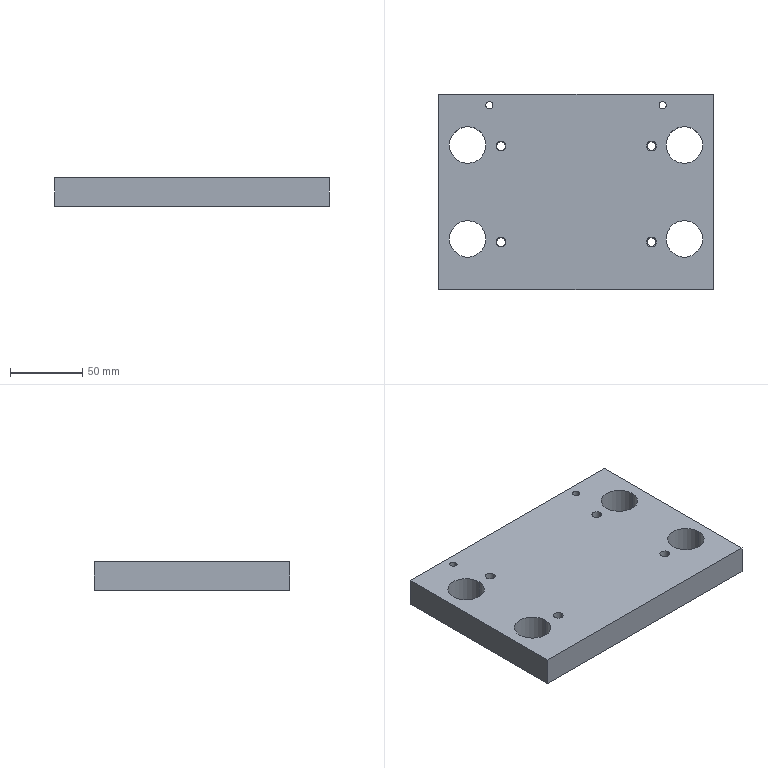Part | SolidWorks | features HoleWzd 2, Extrusion 1 | 1 solid | 34 faces | box 190 x 135 x 20 mm | volume 469337 mm3 | cylinder 20 | cone 8 | plane 6 | commonest cylinder face diameters 6.8 x8 25.224 x8 5 x4
STEP:
#1=CARTESIAN_POINT('',(-55.367,31.821,0.25));
#2=VERTEX_POINT('',#1);
#3=CARTESIAN_POINT('',(-48.567,31.821,0.25));
#4=VERTEX_POINT('',#3);
#5=CARTESIAN_POINT('',(-51.967,31.821,0.25));
#6=DIRECTION('',(0.,0.,1.));
#7=DIRECTION('',(1.,0.,0.));
#8=AXIS2_PLACEMENT_3D('',#5,#6,#7);
#9=CIRCLE('',#8,3.4);
#10=EDGE_CURVE('',#2,#4,#9,.T.);
#11=ORIENTED_EDGE('',*,*,#10,.F.);
#12=CARTESIAN_POINT('',(-55.367,31.821,20.));
#13=VERTEX_POINT('',#12);
#14=CARTESIAN_POINT('',(-55.367,31.821,20.));
#15=DIRECTION('',(0.,0.,1.));
#16=VECTOR('',#15,1000.);
#17=LINE('',#14,#16);
#18=EDGE_CURVE('',#2,#13,#17,.T.);
#19=ORIENTED_EDGE('',*,*,#18,.T.);
#20=CARTESIAN_POINT('',(-48.567,31.821,20.));
#21=VERTEX_POINT('',#20);
#22=CARTESIAN_POINT('',(-51.967,31.821,20.));
#23=DIRECTION('',(0.,0.,1.));
#24=DIRECTION('',(1.,0.,0.));
#25=AXIS2_PLACEMENT_3D('',#22,#23,#24);
#26=CIRCLE('',#25,3.4);
#27=EDGE_CURVE('',#13,#21,#26,.T.);
#28=ORIENTED_EDGE('',*,*,#27,.T.);
#29=CARTESIAN_POINT('',(-48.567,31.821,20.));
#30=DIRECTION('',(0.,0.,1.));
#31=VECTOR('',#30,1000.);
#32=LINE('',#29,#31);
#33=EDGE_CURVE('',#4,#21,#32,.T.);
#34=ORIENTED_EDGE('',*,*,#33,.F.);
#35=EDGE_LOOP('',(#11,#19,#28,#34));
#36=FACE_OUTER_BOUND('',#35,.T.);
#37=CARTESIAN_POINT('',(-51.967,31.821,20.));
#38=DIRECTION('',(0.,0.,1.));
#39=DIRECTION('',(1.,0.,0.));
#40=AXIS2_PLACEMENT_3D('',#37,#38,#39);
#41=CYLINDRICAL_SURFACE('',#40,3.4);
#42=ADVANCED_FACE('',(#36),#41,.F.);
#43=CARTESIAN_POINT('',(-54.951,31.821,0.));
#44=VERTEX_POINT('',#43);
#45=CARTESIAN_POINT('',(-48.984,31.821,0.));
#46=VERTEX_POINT('',#45);
#47=CARTESIAN_POINT('',(-51.967,31.821,0.));
#48=DIRECTION('',(0.,0.,1.));
#49=DIRECTION('',(1.,0.,0.));
#50=AXIS2_PLACEMENT_3D('',#47,#48,#49);
#51=CIRCLE('',#50,2.984);
#52=EDGE_CURVE('',#44,#46,#51,.T.);
#53=ORIENTED_EDGE('',*,*,#52,.F.);
#54=CARTESIAN_POINT('',(-55.367,31.821,0.25));
#55=DIRECTION('',(-0.8572,0.,0.515));
#56=VECTOR('',#55,1000.);
#57=LINE('',#54,#56);
#58=EDGE_CURVE('',#44,#2,#57,.T.);
#59=ORIENTED_EDGE('',*,*,#58,.T.);
#60=ORIENTED_EDGE('',*,*,#10,.T.);
#61=CARTESIAN_POINT('',(-48.567,31.821,0.25));
#62=DIRECTION('',(0.8572,0.,0.515));
#63=VECTOR('',#62,1000.);
#64=LINE('',#61,#63);
#65=EDGE_CURVE('',#46,#4,#64,.T.);
#66=ORIENTED_EDGE('',*,*,#65,.F.);
#67=EDGE_LOOP('',(#53,#59,#60,#66));
#68=FACE_OUTER_BOUND('',#67,.T.);
#69=CARTESIAN_POINT('',(-51.967,31.821,0.25));
#70=DIRECTION('',(0.,0.,1.));
#71=DIRECTION('',(1.,0.,0.));
#72=AXIS2_PLACEMENT_3D('',#69,#70,#71);
#73=CONICAL_SURFACE('',#72,3.4,1.03);
#74=ADVANCED_FACE('',(#68),#73,.F.);
#75=CARTESIAN_POINT('',(-55.367,-34.623,0.25));
#76=VERTEX_POINT('',#75);
#77=CARTESIAN_POINT('',(-48.567,-34.623,0.25));
#78=VERTEX_POINT('',#77);
#79=CARTESIAN_POINT('',(-51.967,-34.623,0.25));
#80=DIRECTION('',(0.,0.,1.));
#81=DIRECTION('',(1.,0.,0.));
#82=AXIS2_PLACEMENT_3D('',#79,#80,#81);
#83=CIRCLE('',#82,3.4);
#84=EDGE_CURVE('',#76,#78,#83,.T.);
#85=ORIENTED_EDGE('',*,*,#84,.F.);
#86=CARTESIAN_POINT('',(-55.367,-34.623,20.));
#87=VERTEX_POINT('',#86);
#88=CARTESIAN_POINT('',(-55.367,-34.623,20.));
#89=DIRECTION('',(0.,0.,1.));
#90=VECTOR('',#89,1000.);
#91=LINE('',#88,#90);
#92=EDGE_CURVE('',#76,#87,#91,.T.);
#93=ORIENTED_EDGE('',*,*,#92,.T.);
#94=CARTESIAN_POINT('',(-48.567,-34.623,20.));
#95=VERTEX_POINT('',#94);
#96=CARTESIAN_POINT('',(-51.967,-34.623,20.));
#97=DIRECTION('',(0.,0.,1.));
#98=DIRECTION('',(1.,0.,0.));
#99=AXIS2_PLACEMENT_3D('',#96,#97,#98);
#100=CIRCLE('',#99,3.4);
#101=EDGE_CURVE('',#87,#95,#100,.T.);
#102=ORIENTED_EDGE('',*,*,#101,.T.);
#103=CARTESIAN_POINT('',(-48.567,-34.623,20.));
#104=DIRECTION('',(0.,0.,1.));
#105=VECTOR('',#104,1000.);
#106=LINE('',#103,#105);
#107=EDGE_CURVE('',#78,#95,#106,.T.);
#108=ORIENTED_EDGE('',*,*,#107,.F.);
#109=EDGE_LOOP('',(#85,#93,#102,#108));
#110=FACE_OUTER_BOUND('',#109,.T.);
#111=CARTESIAN_POINT('',(-51.967,-34.623,20.));
#112=DIRECTION('',(0.,0.,1.));
#113=DIRECTION('',(1.,0.,0.));
#114=AXIS2_PLACEMENT_3D('',#111,#112,#113);
#115=CYLINDRICAL_SURFACE('',#114,3.4);
#116=ADVANCED_FACE('',(#110),#115,.F.);
#117=CARTESIAN_POINT('',(-54.951,-34.623,0.));
#118=VERTEX_POINT('',#117);
#119=CARTESIAN_POINT('',(-48.984,-34.623,0.));
#120=VERTEX_POINT('',#119);
#121=CARTESIAN_POINT('',(-51.967,-34.623,0.));
#122=DIRECTION('',(0.,0.,1.));
#123=DIRECTION('',(1.,0.,0.));
#124=AXIS2_PLACEMENT_3D('',#121,#122,#123);
#125=CIRCLE('',#124,2.984);
#126=EDGE_CURVE('',#118,#120,#125,.T.);
#127=ORIENTED_EDGE('',*,*,#126,.F.);
#128=CARTESIAN_POINT('',(-55.367,-34.623,0.25));
#129=DIRECTION('',(-0.8572,0.,0.515));
#130=VECTOR('',#129,1000.);
#131=LINE('',#128,#130);
#132=EDGE_CURVE('',#118,#76,#131,.T.);
#133=ORIENTED_EDGE('',*,*,#132,.T.);
#134=ORIENTED_EDGE('',*,*,#84,.T.);
#135=CARTESIAN_POINT('',(-48.567,-34.623,0.25));
#136=DIRECTION('',(0.8572,0.,0.515));
#137=VECTOR('',#136,1000.);
#138=LINE('',#135,#137);
#139=EDGE_CURVE('',#120,#78,#138,.T.);
#140=ORIENTED_EDGE('',*,*,#139,.F.);
#141=EDGE_LOOP('',(#127,#133,#134,#140));
#142=FACE_OUTER_BOUND('',#141,.T.);
#143=CARTESIAN_POINT('',(-51.967,-34.623,0.25));
#144=DIRECTION('',(0.,0.,1.));
#145=DIRECTION('',(1.,0.,0.));
#146=AXIS2_PLACEMENT_3D('',#143,#144,#145);
#147=CONICAL_SURFACE('',#146,3.4,1.03);
#148=ADVANCED_FACE('',(#142),#147,.F.);
#149=CARTESIAN_POINT('',(48.834,-34.623,0.25));
#150=VERTEX_POINT('',#149);
#151=CARTESIAN_POINT('',(55.634,-34.623,0.25));
#152=VERTEX_POINT('',#151);
#153=CARTESIAN_POINT('',(52.234,-34.623,0.25));
#154=DIRECTION('',(0.,0.,1.));
#155=DIRECTION('',(1.,0.,0.));
#156=AXIS2_PLACEMENT_3D('',#153,#154,#155);
#157=CIRCLE('',#156,3.4);
#158=EDGE_CURVE('',#150,#152,#157,.T.);
#159=ORIENTED_EDGE('',*,*,#158,.F.);
#160=CARTESIAN_POINT('',(48.834,-34.623,20.));
#161=VERTEX_POINT('',#160);
#162=CARTESIAN_POINT('',(48.834,-34.623,20.));
#163=DIRECTION('',(0.,0.,1.));
#164=VECTOR('',#163,1000.);
#165=LINE('',#162,#164);
#166=EDGE_CURVE('',#150,#161,#165,.T.);
#167=ORIENTED_EDGE('',*,*,#166,.T.);
#168=CARTESIAN_POINT('',(55.634,-34.623,20.));
#169=VERTEX_POINT('',#168);
#170=CARTESIAN_POINT('',(52.234,-34.623,20.));
#171=DIRECTION('',(0.,0.,1.));
#172=DIRECTION('',(1.,0.,0.));
#173=AXIS2_PLACEMENT_3D('',#170,#171,#172);
#174=CIRCLE('',#173,3.4);
#175=EDGE_CURVE('',#161,#169,#174,.T.);
#176=ORIENTED_EDGE('',*,*,#175,.T.);
#177=CARTESIAN_POINT('',(55.634,-34.623,20.));
#178=DIRECTION('',(0.,0.,1.));
#179=VECTOR('',#178,1000.);
#180=LINE('',#177,#179);
#181=EDGE_CURVE('',#152,#169,#180,.T.);
#182=ORIENTED_EDGE('',*,*,#181,.F.);
#183=EDGE_LOOP('',(#159,#167,#176,#182));
#184=FACE_OUTER_BOUND('',#183,.T.);
#185=CARTESIAN_POINT('',(52.234,-34.623,20.));
#186=DIRECTION('',(0.,0.,1.));
#187=DIRECTION('',(1.,0.,0.));
#188=AXIS2_PLACEMENT_3D('',#185,#186,#187);
#189=CYLINDRICAL_SURFACE('',#188,3.4);
#190=ADVANCED_FACE('',(#184),#189,.F.);
#191=CARTESIAN_POINT('',(49.25,-34.623,0.));
#192=VERTEX_POINT('',#191);
#193=CARTESIAN_POINT('',(55.218,-34.623,0.));
#194=VERTEX_POINT('',#193);
#195=CARTESIAN_POINT('',(52.234,-34.623,0.));
#196=DIRECTION('',(0.,0.,1.));
#197=DIRECTION('',(1.,0.,0.));
#198=AXIS2_PLACEMENT_3D('',#195,#196,#197);
#199=CIRCLE('',#198,2.984);
#200=EDGE_CURVE('',#192,#194,#199,.T.);
#201=ORIENTED_EDGE('',*,*,#200,.F.);
#202=CARTESIAN_POINT('',(48.834,-34.623,0.25));
#203=DIRECTION('',(-0.8572,0.,0.515));
#204=VECTOR('',#203,1000.);
#205=LINE('',#202,#204);
#206=EDGE_CURVE('',#192,#150,#205,.T.);
#207=ORIENTED_EDGE('',*,*,#206,.T.);
#208=ORIENTED_EDGE('',*,*,#158,.T.);
#209=CARTESIAN_POINT('',(55.634,-34.623,0.25));
#210=DIRECTION('',(0.8572,0.,0.515));
#211=VECTOR('',#210,1000.);
#212=LINE('',#209,#211);
#213=EDGE_CURVE('',#194,#152,#212,.T.);
#214=ORIENTED_EDGE('',*,*,#213,.F.);
#215=EDGE_LOOP('',(#201,#207,#208,#214));
#216=FACE_OUTER_BOUND('',#215,.T.);
#217=CARTESIAN_POINT('',(52.234,-34.623,0.25));
#218=DIRECTION('',(0.,0.,1.));
#219=DIRECTION('',(1.,0.,0.));
#220=AXIS2_PLACEMENT_3D('',#217,#218,#219);
#221=CONICAL_SURFACE('',#220,3.4,1.03);
#222=ADVANCED_FACE('',(#216),#221,.F.);
#223=CARTESIAN_POINT('',(48.834,31.821,0.25));
#224=VERTEX_POINT('',#223);
#225=CARTESIAN_POINT('',(55.634,31.821,0.25));
#226=VERTEX_POINT('',#225);
#227=CARTESIAN_POINT('',(52.234,31.821,0.25));
#228=DIRECTION('',(0.,0.,1.));
#229=DIRECTION('',(1.,0.,0.));
#230=AXIS2_PLACEMENT_3D('',#227,#228,#229);
#231=CIRCLE('',#230,3.4);
#232=EDGE_CURVE('',#224,#226,#231,.T.);
#233=ORIENTED_EDGE('',*,*,#232,.F.);
#234=CARTESIAN_POINT('',(48.834,31.821,20.));
#235=VERTEX_POINT('',#234);
#236=CARTESIAN_POINT('',(48.834,31.821,20.));
#237=DIRECTION('',(0.,0.,1.));
#238=VECTOR('',#237,1000.);
#239=LINE('',#236,#238);
#240=EDGE_CURVE('',#224,#235,#239,.T.);
#241=ORIENTED_EDGE('',*,*,#240,.T.);
#242=CARTESIAN_POINT('',(55.634,31.821,20.));
#243=VERTEX_POINT('',#242);
#244=CARTESIAN_POINT('',(52.234,31.821,20.));
#245=DIRECTION('',(0.,0.,1.));
#246=DIRECTION('',(1.,0.,0.));
#247=AXIS2_PLACEMENT_3D('',#244,#245,#246);
#248=CIRCLE('',#247,3.4);
#249=EDGE_CURVE('',#235,#243,#248,.T.);
#250=ORIENTED_EDGE('',*,*,#249,.T.);
#251=CARTESIAN_POINT('',(55.634,31.821,20.));
#252=DIRECTION('',(0.,0.,1.));
#253=VECTOR('',#252,1000.);
#254=LINE('',#251,#253);
#255=EDGE_CURVE('',#226,#243,#254,.T.);
#256=ORIENTED_EDGE('',*,*,#255,.F.);
#257=EDGE_LOOP('',(#233,#241,#250,#256));
#258=FACE_OUTER_BOUND('',#257,.T.);
#259=CARTESIAN_POINT('',(52.234,31.821,20.));
#260=DIRECTION('',(0.,0.,1.));
#261=DIRECTION('',(1.,0.,0.));
#262=AXIS2_PLACEMENT_3D('',#259,#260,#261);
#263=CYLINDRICAL_SURFACE('',#262,3.4);
#264=ADVANCED_FACE('',(#258),#263,.F.);
#265=CARTESIAN_POINT('',(49.25,31.821,0.));
#266=VERTEX_POINT('',#265);
#267=CARTESIAN_POINT('',(55.218,31.821,0.));
#268=VERTEX_POINT('',#267);
#269=CARTESIAN_POINT('',(52.234,31.821,0.));
#270=DIRECTION('',(0.,0.,1.));
#271=DIRECTION('',(1.,0.,0.));
#272=AXIS2_PLACEMENT_3D('',#269,#270,#271);
#273=CIRCLE('',#272,2.984);
#274=EDGE_CURVE('',#266,#268,#273,.T.);
#275=ORIENTED_EDGE('',*,*,#274,.F.);
#276=CARTESIAN_POINT('',(48.834,31.821,0.25));
#277=DIRECTION('',(-0.8572,0.,0.515));
#278=VECTOR('',#277,1000.);
#279=LINE('',#276,#278);
#280=EDGE_CURVE('',#266,#224,#279,.T.);
#281=ORIENTED_EDGE('',*,*,#280,.T.);
#282=ORIENTED_EDGE('',*,*,#232,.T.);
#283=CARTESIAN_POINT('',(55.634,31.821,0.25));
#284=DIRECTION('',(0.8572,0.,0.515));
#285=VECTOR('',#284,1000.);
#286=LINE('',#283,#285);
#287=EDGE_CURVE('',#268,#226,#286,.T.);
#288=ORIENTED_EDGE('',*,*,#287,.F.);
#289=EDGE_LOOP('',(#275,#281,#282,#288));
#290=FACE_OUTER_BOUND('',#289,.T.);
#291=CARTESIAN_POINT('',(52.234,31.821,0.25));
#292=DIRECTION('',(0.,0.,1.));
#293=DIRECTION('',(1.,0.,0.));
#294=AXIS2_PLACEMENT_3D('',#291,#292,#293);
#295=CONICAL_SURFACE('',#294,3.4,1.03);
#296=ADVANCED_FACE('',(#290),#295,.F.);
#297=CARTESIAN_POINT('',(62.5,60.,20.));
#298=VERTEX_POINT('',#297);
#299=CARTESIAN_POINT('',(57.5,60.,20.));
#300=VERTEX_POINT('',#299);
#301=CARTESIAN_POINT('',(60.,60.,20.));
#302=DIRECTION('',(0.,0.,-1.));
#303=DIRECTION('',(-1.,0.,0.));
#304=AXIS2_PLACEMENT_3D('',#301,#302,#303);
#305=CIRCLE('',#304,2.5);
#306=EDGE_CURVE('',#298,#300,#305,.T.);
#307=ORIENTED_EDGE('',*,*,#306,.F.);
#308=CARTESIAN_POINT('',(62.5,60.,0.));
#309=VERTEX_POINT('',#308);
#310=CARTESIAN_POINT('',(62.5,60.,0.));
#311=DIRECTION('',(0.,0.,-1.));
#312=VECTOR('',#311,1000.);
#313=LINE('',#310,#312);
#314=EDGE_CURVE('',#298,#309,#313,.T.);
#315=ORIENTED_EDGE('',*,*,#314,.T.);
#316=CARTESIAN_POINT('',(57.5,60.,0.));
#317=VERTEX_POINT('',#316);
#318=CARTESIAN_POINT('',(60.,60.,0.));
#319=DIRECTION('',(0.,0.,-1.));
#320=DIRECTION('',(-1.,0.,0.));
#321=AXIS2_PLACEMENT_3D('',#318,#319,#320);
#322=CIRCLE('',#321,2.5);
#323=EDGE_CURVE('',#309,#317,#322,.T.);
#324=ORIENTED_EDGE('',*,*,#323,.T.);
#325=CARTESIAN_POINT('',(57.5,60.,0.));
#326=DIRECTION('',(0.,0.,-1.));
#327=VECTOR('',#326,1000.);
#328=LINE('',#325,#327);
#329=EDGE_CURVE('',#300,#317,#328,.T.);
#330=ORIENTED_EDGE('',*,*,#329,.F.);
#331=EDGE_LOOP('',(#307,#315,#324,#330));
#332=FACE_OUTER_BOUND('',#331,.T.);
#333=CARTESIAN_POINT('',(60.,60.,0.));
#334=DIRECTION('',(0.,0.,-1.));
#335=DIRECTION('',(-1.,0.,0.));
#336=AXIS2_PLACEMENT_3D('',#333,#334,#335);
#337=CYLINDRICAL_SURFACE('',#336,2.5);
#338=ADVANCED_FACE('',(#332),#337,.F.);
#339=CARTESIAN_POINT('',(-57.5,60.,20.));
#340=VERTEX_POINT('',#339);
#341=CARTESIAN_POINT('',(-62.5,60.,20.));
#342=VERTEX_POINT('',#341);
#343=CARTESIAN_POINT('',(-60.,60.,20.));
#344=DIRECTION('',(0.,0.,-1.));
#345=DIRECTION('',(-1.,0.,0.));
#346=AXIS2_PLACEMENT_3D('',#343,#344,#345);
#347=CIRCLE('',#346,2.5);
#348=EDGE_CURVE('',#340,#342,#347,.T.);
#349=ORIENTED_EDGE('',*,*,#348,.F.);
#350=CARTESIAN_POINT('',(-57.5,60.,0.));
#351=VERTEX_POINT('',#350);
#352=CARTESIAN_POINT('',(-57.5,60.,0.));
#353=DIRECTION('',(0.,0.,-1.));
#354=VECTOR('',#353,1000.);
#355=LINE('',#352,#354);
#356=EDGE_CURVE('',#340,#351,#355,.T.);
#357=ORIENTED_EDGE('',*,*,#356,.T.);
#358=CARTESIAN_POINT('',(-62.5,60.,0.));
#359=VERTEX_POINT('',#358);
#360=CARTESIAN_POINT('',(-60.,60.,0.));
#361=DIRECTION('',(0.,0.,-1.));
#362=DIRECTION('',(-1.,0.,0.));
#363=AXIS2_PLACEMENT_3D('',#360,#361,#362);
#364=CIRCLE('',#363,2.5);
#365=EDGE_CURVE('',#351,#359,#364,.T.);
#366=ORIENTED_EDGE('',*,*,#365,.T.);
#367=CARTESIAN_POINT('',(-62.5,60.,0.));
#368=DIRECTION('',(0.,0.,-1.));
#369=VECTOR('',#368,1000.);
#370=LINE('',#367,#369);
#371=EDGE_CURVE('',#342,#359,#370,.T.);
#372=ORIENTED_EDGE('',*,*,#371,.F.);
#373=EDGE_LOOP('',(#349,#357,#366,#372));
#374=FACE_OUTER_BOUND('',#373,.T.);
#375=CARTESIAN_POINT('',(-60.,60.,0.));
#376=DIRECTION('',(0.,0.,-1.));
#377=DIRECTION('',(-1.,0.,0.));
#378=AXIS2_PLACEMENT_3D('',#375,#376,#377);
#379=CYLINDRICAL_SURFACE('',#378,2.5);
#380=ADVANCED_FACE('',(#374),#379,.F.);
#381=CARTESIAN_POINT('',(62.388,-32.5,20.));
#382=VERTEX_POINT('',#381);
#383=CARTESIAN_POINT('',(87.612,-32.5,20.));
#384=VERTEX_POINT('',#383);
#385=CARTESIAN_POINT('',(75.,-32.5,20.));
#386=DIRECTION('',(0.,0.,1.));
#387=DIRECTION('',(1.,0.,0.));
#388=AXIS2_PLACEMENT_3D('',#385,#386,#387);
#389=CIRCLE('',#388,12.612);
#390=EDGE_CURVE('',#382,#384,#389,.T.);
#391=ORIENTED_EDGE('',*,*,#390,.T.);
#392=CARTESIAN_POINT('',(87.612,-32.5,0.));
#393=VERTEX_POINT('',#392);
#394=CARTESIAN_POINT('',(87.612,-32.5,20.));
#395=DIRECTION('',(0.,0.,-1.));
#396=VECTOR('',#395,1000.);
#397=LINE('',#394,#396);
#398=EDGE_CURVE('',#384,#393,#397,.T.);
#399=ORIENTED_EDGE('',*,*,#398,.T.);
#400=CARTESIAN_POINT('',(62.388,-32.5,0.));
#401=VERTEX_POINT('',#400);
#402=CARTESIAN_POINT('',(75.,-32.5,0.));
#403=DIRECTION('',(0.,0.,1.));
#404=DIRECTION('',(1.,0.,0.));
#405=AXIS2_PLACEMENT_3D('',#402,#403,#404);
#406=CIRCLE('',#405,12.612);
#407=EDGE_CURVE('',#401,#393,#406,.T.);
#408=ORIENTED_EDGE('',*,*,#407,.F.);
#409=CARTESIAN_POINT('',(62.388,-32.5,20.));
#410=DIRECTION('',(0.,0.,-1.));
#411=VECTOR('',#410,1000.);
#412=LINE('',#409,#411);
#413=EDGE_CURVE('',#382,#401,#412,.T.);
#414=ORIENTED_EDGE('',*,*,#413,.F.);
#415=EDGE_LOOP('',(#391,#399,#408,#414));
#416=FACE_OUTER_BOUND('',#415,.T.);
#417=CARTESIAN_POINT('',(75.,-32.5,20.));
#418=DIRECTION('',(0.,0.,-1.));
#419=DIRECTION('',(-1.,0.,0.));
#420=AXIS2_PLACEMENT_3D('',#417,#418,#419);
#421=CYLINDRICAL_SURFACE('',#420,12.612);
#422=ADVANCED_FACE('',(#416),#421,.F.);
#423=CARTESIAN_POINT('',(62.388,32.5,20.));
#424=VERTEX_POINT('',#423);
#425=CARTESIAN_POINT('',(87.612,32.5,20.));
#426=VERTEX_POINT('',#425);
#427=CARTESIAN_POINT('',(75.,32.5,20.));
#428=DIRECTION('',(0.,0.,1.));
#429=DIRECTION('',(1.,0.,0.));
#430=AXIS2_PLACEMENT_3D('',#427,#428,#429);
#431=CIRCLE('',#430,12.612);
#432=EDGE_CURVE('',#424,#426,#431,.T.);
#433=ORIENTED_EDGE('',*,*,#432,.T.);
#434=CARTESIAN_POINT('',(87.612,32.5,0.));
#435=VERTEX_POINT('',#434);
#436=CARTESIAN_POINT('',(87.612,32.5,20.));
#437=DIRECTION('',(0.,0.,-1.));
#438=VECTOR('',#437,1000.);
#439=LINE('',#436,#438);
#440=EDGE_CURVE('',#426,#435,#439,.T.);
#441=ORIENTED_EDGE('',*,*,#440,.T.);
#442=CARTESIAN_POINT('',(62.388,32.5,0.));
#443=VERTEX_POINT('',#442);
#444=CARTESIAN_POINT('',(75.,32.5,0.));
#445=DIRECTION('',(0.,0.,1.));
#446=DIRECTION('',(1.,0.,0.));
#447=AXIS2_PLACEMENT_3D('',#444,#445,#446);
#448=CIRCLE('',#447,12.612);
#449=EDGE_CURVE('',#443,#435,#448,.T.);
#450=ORIENTED_EDGE('',*,*,#449,.F.);
#451=CARTESIAN_POINT('',(62.388,32.5,20.));
#452=DIRECTION('',(0.,0.,-1.));
#453=VECTOR('',#452,1000.);
#454=LINE('',#451,#453);
#455=EDGE_CURVE('',#424,#443,#454,.T.);
#456=ORIENTED_EDGE('',*,*,#455,.F.);
#457=EDGE_LOOP('',(#433,#441,#450,#456));
#458=FACE_OUTER_BOUND('',#457,.T.);
#459=CARTESIAN_POINT('',(75.,32.5,20.));
#460=DIRECTION('',(0.,0.,-1.));
#461=DIRECTION('',(-1.,0.,0.));
#462=AXIS2_PLACEMENT_3D('',#459,#460,#461);
#463=CYLINDRICAL_SURFACE('',#462,12.612);
#464=ADVANCED_FACE('',(#458),#463,.F.);
#465=CARTESIAN_POINT('',(-87.612,-32.5,20.));
#466=VERTEX_POINT('',#465);
#467=CARTESIAN_POINT('',(-62.388,-32.5,20.));
#468=VERTEX_POINT('',#467);
#469=CARTESIAN_POINT('',(-75.,-32.5,20.));
#470=DIRECTION('',(0.,0.,1.));
#471=DIRECTION('',(1.,0.,0.));
#472=AXIS2_PLACEMENT_3D('',#469,#470,#471);
#473=CIRCLE('',#472,12.612);
#474=EDGE_CURVE('',#466,#468,#473,.T.);
#475=ORIENTED_EDGE('',*,*,#474,.T.);
#476=CARTESIAN_POINT('',(-62.388,-32.5,0.));
#477=VERTEX_POINT('',#476);
#478=CARTESIAN_POINT('',(-62.388,-32.5,20.));
#479=DIRECTION('',(0.,0.,-1.));
#480=VECTOR('',#479,1000.);
#481=LINE('',#478,#480);
#482=EDGE_CURVE('',#468,#477,#481,.T.);
#483=ORIENTED_EDGE('',*,*,#482,.T.);
#484=CARTESIAN_POINT('',(-87.612,-32.5,0.));
#485=VERTEX_POINT('',#484);
#486=CARTESIAN_POINT('',(-75.,-32.5,0.));
#487=DIRECTION('',(0.,0.,1.));
#488=DIRECTION('',(1.,0.,0.));
#489=AXIS2_PLACEMENT_3D('',#486,#487,#488);
#490=CIRCLE('',#489,12.612);
#491=EDGE_CURVE('',#485,#477,#490,.T.);
#492=ORIENTED_EDGE('',*,*,#491,.F.);
#493=CARTESIAN_POINT('',(-87.612,-32.5,20.));
#494=DIRECTION('',(0.,0.,-1.));
#495=VECTOR('',#494,1000.);
#496=LINE('',#493,#495);
#497=EDGE_CURVE('',#466,#485,#496,.T.);
#498=ORIENTED_EDGE('',*,*,#497,.F.);
#499=EDGE_LOOP('',(#475,#483,#492,#498));
#500=FACE_OUTER_BOUND('',#499,.T.);
#501=CARTESIAN_POINT('',(-75.,-32.5,20.));
#502=DIRECTION('',(0.,0.,-1.));
#503=DIRECTION('',(-1.,0.,0.));
#504=AXIS2_PLACEMENT_3D('',#501,#502,#503);
#505=CYLINDRICAL_SURFACE('',#504,12.612);
#506=ADVANCED_FACE('',(#500),#505,.F.);
#507=CARTESIAN_POINT('',(-87.612,32.5,20.));
#508=VERTEX_POINT('',#507);
#509=CARTESIAN_POINT('',(-62.388,32.5,20.));
#510=VERTEX_POINT('',#509);
#511=CARTESIAN_POINT('',(-75.,32.5,20.));
#512=DIRECTION('',(0.,0.,1.));
#513=DIRECTION('',(1.,0.,0.));
#514=AXIS2_PLACEMENT_3D('',#511,#512,#513);
#515=CIRCLE('',#514,12.612);
#516=EDGE_CURVE('',#508,#510,#515,.T.);
#517=ORIENTED_EDGE('',*,*,#516,.T.);
#518=CARTESIAN_POINT('',(-62.388,32.5,0.));
#519=VERTEX_POINT('',#518);
#520=CARTESIAN_POINT('',(-62.388,32.5,20.));
#521=DIRECTION('',(0.,0.,-1.));
#522=VECTOR('',#521,1000.);
#523=LINE('',#520,#522);
#524=EDGE_CURVE('',#510,#519,#523,.T.);
#525=ORIENTED_EDGE('',*,*,#524,.T.);
#526=CARTESIAN_POINT('',(-87.612,32.5,0.));
#527=VERTEX_POINT('',#526);
#528=CARTESIAN_POINT('',(-75.,32.5,0.));
#529=DIRECTION('',(0.,0.,1.));
#530=DIRECTION('',(1.,0.,0.));
#531=AXIS2_PLACEMENT_3D('',#528,#529,#530);
#532=CIRCLE('',#531,12.612);
#533=EDGE_CURVE('',#527,#519,#532,.T.);
#534=ORIENTED_EDGE('',*,*,#533,.F.);
#535=CARTESIAN_POINT('',(-87.612,32.5,20.));
#536=DIRECTION('',(0.,0.,-1.));
#537=VECTOR('',#536,1000.);
#538=LINE('',#535,#537);
#539=EDGE_CURVE('',#508,#527,#538,.T.);
#540=ORIENTED_EDGE('',*,*,#539,.F.);
#541=EDGE_LOOP('',(#517,#525,#534,#540));
#542=FACE_OUTER_BOUND('',#541,.T.);
#543=CARTESIAN_POINT('',(-75.,32.5,20.));
#544=DIRECTION('',(0.,0.,-1.));
#545=DIRECTION('',(-1.,0.,0.));
#546=AXIS2_PLACEMENT_3D('',#543,#544,#545);
#547=CYLINDRICAL_SURFACE('',#546,12.612);
#548=ADVANCED_FACE('',(#542),#547,.F.);
#549=CARTESIAN_POINT('',(-51.967,31.821,20.));
#550=DIRECTION('',(0.,0.,1.));
#551=DIRECTION('',(1.,0.,0.));
#552=AXIS2_PLACEMENT_3D('',#549,#550,#551);
#553=CIRCLE('',#552,3.4);
#554=EDGE_CURVE('',#21,#13,#553,.T.);
#555=ORIENTED_EDGE('',*,*,#554,.F.);
#556=ORIENTED_EDGE('',*,*,#27,.F.);
#557=EDGE_LOOP('',(#555,#556));
#558=FACE_BOUND('',#557,.T.);
#559=CARTESIAN_POINT('',(-51.967,-34.623,20.));
#560=DIRECTION('',(0.,0.,1.));
#561=DIRECTION('',(1.,0.,0.));
#562=AXIS2_PLACEMENT_3D('',#559,#560,#561);
#563=CIRCLE('',#562,3.4);
#564=EDGE_CURVE('',#95,#87,#563,.T.);
#565=ORIENTED_EDGE('',*,*,#564,.F.);
#566=ORIENTED_EDGE('',*,*,#101,.F.);
#567=EDGE_LOOP('',(#565,#566));
#568=FACE_BOUND('',#567,.T.);
#569=CARTESIAN_POINT('',(52.234,-34.623,20.));
#570=DIRECTION('',(0.,0.,1.));
#571=DIRECTION('',(1.,0.,0.));
#572=AXIS2_PLACEMENT_3D('',#569,#570,#571);
#573=CIRCLE('',#572,3.4);
#574=EDGE_CURVE('',#169,#161,#573,.T.);
#575=ORIENTED_EDGE('',*,*,#574,.F.);
#576=ORIENTED_EDGE('',*,*,#175,.F.);
#577=EDGE_LOOP('',(#575,#576));
#578=FACE_BOUND('',#577,.T.);
#579=CARTESIAN_POINT('',(52.234,31.821,20.));
#580=DIRECTION('',(0.,0.,1.));
#581=DIRECTION('',(1.,0.,0.));
#582=AXIS2_PLACEMENT_3D('',#579,#580,#581);
#583=CIRCLE('',#582,3.4);
#584=EDGE_CURVE('',#243,#235,#583,.T.);
#585=ORIENTED_EDGE('',*,*,#584,.F.);
#586=ORIENTED_EDGE('',*,*,#249,.F.);
#587=EDGE_LOOP('',(#585,#586));
#588=FACE_BOUND('',#587,.T.);
#589=CARTESIAN_POINT('',(60.,60.,20.));
#590=DIRECTION('',(0.,0.,-1.));
#591=DIRECTION('',(-1.,0.,0.));
#592=AXIS2_PLACEMENT_3D('',#589,#590,#591);
#593=CIRCLE('',#592,2.5);
#594=EDGE_CURVE('',#300,#298,#593,.T.);
#595=ORIENTED_EDGE('',*,*,#594,.T.);
#596=ORIENTED_EDGE('',*,*,#306,.T.);
#597=EDGE_LOOP('',(#595,#596));
#598=FACE_BOUND('',#597,.T.);
#599=CARTESIAN_POINT('',(-60.,60.,20.));
#600=DIRECTION('',(0.,0.,-1.));
#601=DIRECTION('',(-1.,0.,0.));
#602=AXIS2_PLACEMENT_3D('',#599,#600,#601);
#603=CIRCLE('',#602,2.5);
#604=EDGE_CURVE('',#342,#340,#603,.T.);
#605=ORIENTED_EDGE('',*,*,#604,.T.);
#606=ORIENTED_EDGE('',*,*,#348,.T.);
#607=EDGE_LOOP('',(#605,#606));
#608=FACE_BOUND('',#607,.T.);
#609=ORIENTED_EDGE('',*,*,#432,.F.);
#610=CARTESIAN_POINT('',(75.,32.5,20.));
#611=DIRECTION('',(0.,0.,1.));
#612=DIRECTION('',(1.,0.,0.));
#613=AXIS2_PLACEMENT_3D('',#610,#611,#612);
#614=CIRCLE('',#613,12.612);
#615=EDGE_CURVE('',#426,#424,#614,.T.);
#616=ORIENTED_EDGE('',*,*,#615,.F.);
#617=EDGE_LOOP('',(#609,#616));
#618=FACE_BOUND('',#617,.T.);
#619=ORIENTED_EDGE('',*,*,#516,.F.);
#620=CARTESIAN_POINT('',(-75.,32.5,20.));
#621=DIRECTION('',(0.,0.,1.));
#622=DIRECTION('',(1.,0.,0.));
#623=AXIS2_PLACEMENT_3D('',#620,#621,#622);
#624=CIRCLE('',#623,12.612);
#625=EDGE_CURVE('',#510,#508,#624,.T.);
#626=ORIENTED_EDGE('',*,*,#625,.F.);
#627=EDGE_LOOP('',(#619,#626));
#628=FACE_BOUND('',#627,.T.);
#629=CARTESIAN_POINT('',(95.,-67.5,20.));
#630=VERTEX_POINT('',#629);
#631=CARTESIAN_POINT('',(95.,67.5,20.));
#632=VERTEX_POINT('',#631);
#633=CARTESIAN_POINT('',(95.,67.5,20.));
#634=DIRECTION('',(0.,1.,0.));
#635=VECTOR('',#634,1000.);
#636=LINE('',#633,#635);
#637=EDGE_CURVE('',#630,#632,#636,.T.);
#638=ORIENTED_EDGE('',*,*,#637,.T.);
#639=CARTESIAN_POINT('',(-95.,67.5,20.));
#640=VERTEX_POINT('',#639);
#641=CARTESIAN_POINT('',(-95.,67.5,20.));
#642=DIRECTION('',(-1.,0.,0.));
#643=VECTOR('',#642,1000.);
#644=LINE('',#641,#643);
#645=EDGE_CURVE('',#632,#640,#644,.T.);
#646=ORIENTED_EDGE('',*,*,#645,.T.);
#647=CARTESIAN_POINT('',(-95.,-67.5,20.));
#648=VERTEX_POINT('',#647);
#649=CARTESIAN_POINT('',(-95.,67.5,20.));
#650=DIRECTION('',(0.,-1.,0.));
#651=VECTOR('',#650,1000.);
#652=LINE('',#649,#651);
#653=EDGE_CURVE('',#640,#648,#652,.T.);
#654=ORIENTED_EDGE('',*,*,#653,.T.);
#655=CARTESIAN_POINT('',(-95.,-67.5,20.));
#656=DIRECTION('',(1.,0.,0.));
#657=VECTOR('',#656,1000.);
#658=LINE('',#655,#657);
#659=EDGE_CURVE('',#648,#630,#658,.T.);
#660=ORIENTED_EDGE('',*,*,#659,.T.);
#661=EDGE_LOOP('',(#638,#646,#654,#660));
#662=FACE_OUTER_BOUND('',#661,.T.);
#663=ORIENTED_EDGE('',*,*,#474,.F.);
#664=CARTESIAN_POINT('',(-75.,-32.5,20.));
#665=DIRECTION('',(0.,0.,1.));
#666=DIRECTION('',(1.,0.,0.));
#667=AXIS2_PLACEMENT_3D('',#664,#665,#666);
#668=CIRCLE('',#667,12.612);
#669=EDGE_CURVE('',#468,#466,#668,.T.);
#670=ORIENTED_EDGE('',*,*,#669,.F.);
#671=EDGE_LOOP('',(#663,#670));
#672=FACE_BOUND('',#671,.T.);
#673=ORIENTED_EDGE('',*,*,#390,.F.);
#674=CARTESIAN_POINT('',(75.,-32.5,20.));
#675=DIRECTION('',(0.,0.,1.));
#676=DIRECTION('',(1.,0.,0.));
#677=AXIS2_PLACEMENT_3D('',#674,#675,#676);
#678=CIRCLE('',#677,12.612);
#679=EDGE_CURVE('',#384,#382,#678,.T.);
#680=ORIENTED_EDGE('',*,*,#679,.F.);
#681=EDGE_LOOP('',(#673,#680));
#682=FACE_BOUND('',#681,.T.);
#683=CARTESIAN_POINT('',(0.,0.,20.));
#684=DIRECTION('',(0.,0.,1.));
#685=DIRECTION('',(1.,0.,0.));
#686=AXIS2_PLACEMENT_3D('',#683,#684,#685);
#687=PLANE('',#686);
#688=ADVANCED_FACE('',(#558,#568,#578,#588,#598,#608,#618,#628,#662,#672,#682),#687,.T.);
#689=CARTESIAN_POINT('',(-51.967,31.821,0.));
#690=DIRECTION('',(0.,0.,1.));
#691=DIRECTION('',(1.,0.,0.));
#692=AXIS2_PLACEMENT_3D('',#689,#690,#691);
#693=CIRCLE('',#692,2.984);
#694=EDGE_CURVE('',#46,#44,#693,.T.);
#695=ORIENTED_EDGE('',*,*,#694,.T.);
#696=ORIENTED_EDGE('',*,*,#52,.T.);
#697=EDGE_LOOP('',(#695,#696));
#698=FACE_BOUND('',#697,.T.);
#699=CARTESIAN_POINT('',(-51.967,-34.623,0.));
#700=DIRECTION('',(0.,0.,1.));
#701=DIRECTION('',(1.,0.,0.));
#702=AXIS2_PLACEMENT_3D('',#699,#700,#701);
#703=CIRCLE('',#702,2.984);
#704=EDGE_CURVE('',#120,#118,#703,.T.);
#705=ORIENTED_EDGE('',*,*,#704,.T.);
#706=ORIENTED_EDGE('',*,*,#126,.T.);
#707=EDGE_LOOP('',(#705,#706));
#708=FACE_BOUND('',#707,.T.);
#709=CARTESIAN_POINT('',(52.234,-34.623,0.));
#710=DIRECTION('',(0.,0.,1.));
#711=DIRECTION('',(1.,0.,0.));
#712=AXIS2_PLACEMENT_3D('',#709,#710,#711);
#713=CIRCLE('',#712,2.984);
#714=EDGE_CURVE('',#194,#192,#713,.T.);
#715=ORIENTED_EDGE('',*,*,#714,.T.);
#716=ORIENTED_EDGE('',*,*,#200,.T.);
#717=EDGE_LOOP('',(#715,#716));
#718=FACE_BOUND('',#717,.T.);
#719=CARTESIAN_POINT('',(52.234,31.821,0.));
#720=DIRECTION('',(0.,0.,1.));
#721=DIRECTION('',(1.,0.,0.));
#722=AXIS2_PLACEMENT_3D('',#719,#720,#721);
#723=CIRCLE('',#722,2.984);
#724=EDGE_CURVE('',#268,#266,#723,.T.);
#725=ORIENTED_EDGE('',*,*,#724,.T.);
#726=ORIENTED_EDGE('',*,*,#274,.T.);
#727=EDGE_LOOP('',(#725,#726));
#728=FACE_BOUND('',#727,.T.);
#729=CARTESIAN_POINT('',(60.,60.,0.));
#730=DIRECTION('',(0.,0.,-1.));
#731=DIRECTION('',(-1.,0.,0.));
#732=AXIS2_PLACEMENT_3D('',#729,#730,#731);
#733=CIRCLE('',#732,2.5);
#734=EDGE_CURVE('',#317,#309,#733,.T.);
#735=ORIENTED_EDGE('',*,*,#734,.F.);
#736=ORIENTED_EDGE('',*,*,#323,.F.);
#737=EDGE_LOOP('',(#735,#736));
#738=FACE_BOUND('',#737,.T.);
#739=CARTESIAN_POINT('',(-60.,60.,0.));
#740=DIRECTION('',(0.,0.,-1.));
#741=DIRECTION('',(-1.,0.,0.));
#742=AXIS2_PLACEMENT_3D('',#739,#740,#741);
#743=CIRCLE('',#742,2.5);
#744=EDGE_CURVE('',#359,#351,#743,.T.);
#745=ORIENTED_EDGE('',*,*,#744,.F.);
#746=ORIENTED_EDGE('',*,*,#365,.F.);
#747=EDGE_LOOP('',(#745,#746));
#748=FACE_BOUND('',#747,.T.);
#749=CARTESIAN_POINT('',(95.,-67.5,0.));
#750=VERTEX_POINT('',#749);
#751=CARTESIAN_POINT('',(95.,67.5,0.));
#752=VERTEX_POINT('',#751);
#753=CARTESIAN_POINT('',(95.,67.5,0.));
#754=DIRECTION('',(0.,1.,0.));
#755=VECTOR('',#754,1000.);
#756=LINE('',#753,#755);
#757=EDGE_CURVE('',#750,#752,#756,.T.);
#758=ORIENTED_EDGE('',*,*,#757,.F.);
#759=CARTESIAN_POINT('',(-95.,-67.5,0.));
#760=VERTEX_POINT('',#759);
#761=CARTESIAN_POINT('',(-95.,-67.5,0.));
#762=DIRECTION('',(1.,0.,0.));
#763=VECTOR('',#762,1000.);
#764=LINE('',#761,#763);
#765=EDGE_CURVE('',#760,#750,#764,.T.);
#766=ORIENTED_EDGE('',*,*,#765,.F.);
#767=CARTESIAN_POINT('',(-95.,67.5,0.));
#768=VERTEX_POINT('',#767);
#769=CARTESIAN_POINT('',(-95.,67.5,0.));
#770=DIRECTION('',(0.,-1.,0.));
#771=VECTOR('',#770,1000.);
#772=LINE('',#769,#771);
#773=EDGE_CURVE('',#768,#760,#772,.T.);
#774=ORIENTED_EDGE('',*,*,#773,.F.);
#775=CARTESIAN_POINT('',(-95.,67.5,0.));
#776=DIRECTION('',(-1.,0.,0.));
#777=VECTOR('',#776,1000.);
#778=LINE('',#775,#777);
#779=EDGE_CURVE('',#752,#768,#778,.T.);
#780=ORIENTED_EDGE('',*,*,#779,.F.);
#781=EDGE_LOOP('',(#758,#766,#774,#780));
#782=FACE_OUTER_BOUND('',#781,.T.);
#783=ORIENTED_EDGE('',*,*,#533,.T.);
#784=CARTESIAN_POINT('',(-75.,32.5,0.));
#785=DIRECTION('',(0.,0.,1.));
#786=DIRECTION('',(1.,0.,0.));
#787=AXIS2_PLACEMENT_3D('',#784,#785,#786);
#788=CIRCLE('',#787,12.612);
#789=EDGE_CURVE('',#519,#527,#788,.T.);
#790=ORIENTED_EDGE('',*,*,#789,.T.);
#791=EDGE_LOOP('',(#783,#790));
#792=FACE_BOUND('',#791,.T.);
#793=ORIENTED_EDGE('',*,*,#491,.T.);
#794=CARTESIAN_POINT('',(-75.,-32.5,0.));
#795=DIRECTION('',(0.,0.,1.));
#796=DIRECTION('',(1.,0.,0.));
#797=AXIS2_PLACEMENT_3D('',#794,#795,#796);
#798=CIRCLE('',#797,12.612);
#799=EDGE_CURVE('',#477,#485,#798,.T.);
#800=ORIENTED_EDGE('',*,*,#799,.T.);
#801=EDGE_LOOP('',(#793,#800));
#802=FACE_BOUND('',#801,.T.);
#803=ORIENTED_EDGE('',*,*,#449,.T.);
#804=CARTESIAN_POINT('',(75.,32.5,0.));
#805=DIRECTION('',(0.,0.,1.));
#806=DIRECTION('',(1.,0.,0.));
#807=AXIS2_PLACEMENT_3D('',#804,#805,#806);
#808=CIRCLE('',#807,12.612);
#809=EDGE_CURVE('',#435,#443,#808,.T.);
#810=ORIENTED_EDGE('',*,*,#809,.T.);
#811=EDGE_LOOP('',(#803,#810));
#812=FACE_BOUND('',#811,.T.);
#813=ORIENTED_EDGE('',*,*,#407,.T.);
#814=CARTESIAN_POINT('',(75.,-32.5,0.));
#815=DIRECTION('',(0.,0.,1.));
#816=DIRECTION('',(1.,0.,0.));
#817=AXIS2_PLACEMENT_3D('',#814,#815,#816);
#818=CIRCLE('',#817,12.612);
#819=EDGE_CURVE('',#393,#401,#818,.T.);
#820=ORIENTED_EDGE('',*,*,#819,.T.);
#821=EDGE_LOOP('',(#813,#820));
#822=FACE_BOUND('',#821,.T.);
#823=CARTESIAN_POINT('',(0.,0.,0.));
#824=DIRECTION('',(0.,0.,1.));
#825=DIRECTION('',(1.,0.,0.));
#826=AXIS2_PLACEMENT_3D('',#823,#824,#825);
#827=PLANE('',#826);
#828=ADVANCED_FACE('',(#698,#708,#718,#728,#738,#748,#782,#792,#802,#812,#822),#827,.F.);
#829=ORIENTED_EDGE('',*,*,#757,.T.);
#830=CARTESIAN_POINT('',(95.,67.5,20.));
#831=DIRECTION('',(0.,0.,-1.));
#832=VECTOR('',#831,1000.);
#833=LINE('',#830,#832);
#834=EDGE_CURVE('',#632,#752,#833,.T.);
#835=ORIENTED_EDGE('',*,*,#834,.F.);
#836=ORIENTED_EDGE('',*,*,#637,.F.);
#837=CARTESIAN_POINT('',(95.,-67.5,20.));
#838=DIRECTION('',(0.,0.,-1.));
#839=VECTOR('',#838,1000.);
#840=LINE('',#837,#839);
#841=EDGE_CURVE('',#630,#750,#840,.T.);
#842=ORIENTED_EDGE('',*,*,#841,.T.);
#843=EDGE_LOOP('',(#829,#835,#836,#842));
#844=FACE_OUTER_BOUND('',#843,.T.);
#845=CARTESIAN_POINT('',(95.,67.5,20.));
#846=DIRECTION('',(-1.,0.,0.));
#847=DIRECTION('',(0.,-1.,0.));
#848=AXIS2_PLACEMENT_3D('',#845,#846,#847);
#849=PLANE('',#848);
#850=ADVANCED_FACE('',(#844),#849,.F.);
#851=ORIENTED_EDGE('',*,*,#779,.T.);
#852=CARTESIAN_POINT('',(-95.,67.5,20.));
#853=DIRECTION('',(0.,0.,-1.));
#854=VECTOR('',#853,1000.);
#855=LINE('',#852,#854);
#856=EDGE_CURVE('',#640,#768,#855,.T.);
#857=ORIENTED_EDGE('',*,*,#856,.F.);
#858=ORIENTED_EDGE('',*,*,#645,.F.);
#859=ORIENTED_EDGE('',*,*,#834,.T.);
#860=EDGE_LOOP('',(#851,#857,#858,#859));
#861=FACE_OUTER_BOUND('',#860,.T.);
#862=CARTESIAN_POINT('',(-95.,67.5,20.));
#863=DIRECTION('',(0.,-1.,0.));
#864=DIRECTION('',(0.,0.,-1.));
#865=AXIS2_PLACEMENT_3D('',#862,#863,#864);
#866=PLANE('',#865);
#867=ADVANCED_FACE('',(#861),#866,.F.);
#868=ORIENTED_EDGE('',*,*,#773,.T.);
#869=CARTESIAN_POINT('',(-95.,-67.5,20.));
#870=DIRECTION('',(0.,0.,-1.));
#871=VECTOR('',#870,1000.);
#872=LINE('',#869,#871);
#873=EDGE_CURVE('',#648,#760,#872,.T.);
#874=ORIENTED_EDGE('',*,*,#873,.F.);
#875=ORIENTED_EDGE('',*,*,#653,.F.);
#876=ORIENTED_EDGE('',*,*,#856,.T.);
#877=EDGE_LOOP('',(#868,#874,#875,#876));
#878=FACE_OUTER_BOUND('',#877,.T.);
#879=CARTESIAN_POINT('',(-95.,67.5,20.));
#880=DIRECTION('',(1.,0.,0.));
#881=DIRECTION('',(0.,1.,0.));
#882=AXIS2_PLACEMENT_3D('',#879,#880,#881);
#883=PLANE('',#882);
#884=ADVANCED_FACE('',(#878),#883,.F.);
#885=ORIENTED_EDGE('',*,*,#765,.T.);
#886=ORIENTED_EDGE('',*,*,#841,.F.);
#887=ORIENTED_EDGE('',*,*,#659,.F.);
#888=ORIENTED_EDGE('',*,*,#873,.T.);
#889=EDGE_LOOP('',(#885,#886,#887,#888));
#890=FACE_OUTER_BOUND('',#889,.T.);
#891=CARTESIAN_POINT('',(-95.,-67.5,20.));
#892=DIRECTION('',(0.,1.,0.));
#893=DIRECTION('',(0.,0.,1.));
#894=AXIS2_PLACEMENT_3D('',#891,#892,#893);
#895=PLANE('',#894);
#896=ADVANCED_FACE('',(#890),#895,.F.);
#897=ORIENTED_EDGE('',*,*,#524,.F.);
#898=ORIENTED_EDGE('',*,*,#625,.T.);
#899=ORIENTED_EDGE('',*,*,#539,.T.);
#900=ORIENTED_EDGE('',*,*,#789,.F.);
#901=EDGE_LOOP('',(#897,#898,#899,#900));
#902=FACE_OUTER_BOUND('',#901,.T.);
#903=CARTESIAN_POINT('',(-75.,32.5,20.));
#904=DIRECTION('',(0.,0.,-1.));
#905=DIRECTION('',(-1.,0.,0.));
#906=AXIS2_PLACEMENT_3D('',#903,#904,#905);
#907=CYLINDRICAL_SURFACE('',#906,12.612);
#908=ADVANCED_FACE('',(#902),#907,.F.);
#909=ORIENTED_EDGE('',*,*,#482,.F.);
#910=ORIENTED_EDGE('',*,*,#669,.T.);
#911=ORIENTED_EDGE('',*,*,#497,.T.);
#912=ORIENTED_EDGE('',*,*,#799,.F.);
#913=EDGE_LOOP('',(#909,#910,#911,#912));
#914=FACE_OUTER_BOUND('',#913,.T.);
#915=CARTESIAN_POINT('',(-75.,-32.5,20.));
#916=DIRECTION('',(0.,0.,-1.));
#917=DIRECTION('',(-1.,0.,0.));
#918=AXIS2_PLACEMENT_3D('',#915,#916,#917);
#919=CYLINDRICAL_SURFACE('',#918,12.612);
#920=ADVANCED_FACE('',(#914),#919,.F.);
#921=ORIENTED_EDGE('',*,*,#440,.F.);
#922=ORIENTED_EDGE('',*,*,#615,.T.);
#923=ORIENTED_EDGE('',*,*,#455,.T.);
#924=ORIENTED_EDGE('',*,*,#809,.F.);
#925=EDGE_LOOP('',(#921,#922,#923,#924));
#926=FACE_OUTER_BOUND('',#925,.T.);
#927=CARTESIAN_POINT('',(75.,32.5,20.));
#928=DIRECTION('',(0.,0.,-1.));
#929=DIRECTION('',(-1.,0.,0.));
#930=AXIS2_PLACEMENT_3D('',#927,#928,#929);
#931=CYLINDRICAL_SURFACE('',#930,12.612);
#932=ADVANCED_FACE('',(#926),#931,.F.);
#933=ORIENTED_EDGE('',*,*,#398,.F.);
#934=ORIENTED_EDGE('',*,*,#679,.T.);
#935=ORIENTED_EDGE('',*,*,#413,.T.);
#936=ORIENTED_EDGE('',*,*,#819,.F.);
#937=EDGE_LOOP('',(#933,#934,#935,#936));
#938=FACE_OUTER_BOUND('',#937,.T.);
#939=CARTESIAN_POINT('',(75.,-32.5,20.));
#940=DIRECTION('',(0.,0.,-1.));
#941=DIRECTION('',(-1.,0.,0.));
#942=AXIS2_PLACEMENT_3D('',#939,#940,#941);
#943=CYLINDRICAL_SURFACE('',#942,12.612);
#944=ADVANCED_FACE('',(#938),#943,.F.);
#945=ORIENTED_EDGE('',*,*,#356,.F.);
#946=ORIENTED_EDGE('',*,*,#604,.F.);
#947=ORIENTED_EDGE('',*,*,#371,.T.);
#948=ORIENTED_EDGE('',*,*,#744,.T.);
#949=EDGE_LOOP('',(#945,#946,#947,#948));
#950=FACE_OUTER_BOUND('',#949,.T.);
#951=CARTESIAN_POINT('',(-60.,60.,0.));
#952=DIRECTION('',(0.,0.,-1.));
#953=DIRECTION('',(-1.,0.,0.));
#954=AXIS2_PLACEMENT_3D('',#951,#952,#953);
#955=CYLINDRICAL_SURFACE('',#954,2.5);
#956=ADVANCED_FACE('',(#950),#955,.F.);
#957=ORIENTED_EDGE('',*,*,#314,.F.);
#958=ORIENTED_EDGE('',*,*,#594,.F.);
#959=ORIENTED_EDGE('',*,*,#329,.T.);
#960=ORIENTED_EDGE('',*,*,#734,.T.);
#961=EDGE_LOOP('',(#957,#958,#959,#960));
#962=FACE_OUTER_BOUND('',#961,.T.);
#963=CARTESIAN_POINT('',(60.,60.,0.));
#964=DIRECTION('',(0.,0.,-1.));
#965=DIRECTION('',(-1.,0.,0.));
#966=AXIS2_PLACEMENT_3D('',#963,#964,#965);
#967=CYLINDRICAL_SURFACE('',#966,2.5);
#968=ADVANCED_FACE('',(#962),#967,.F.);
#969=ORIENTED_EDGE('',*,*,#280,.F.);
#970=ORIENTED_EDGE('',*,*,#724,.F.);
#971=ORIENTED_EDGE('',*,*,#287,.T.);
#972=CARTESIAN_POINT('',(52.234,31.821,0.25));
#973=DIRECTION('',(0.,0.,1.));
#974=DIRECTION('',(1.,0.,0.));
#975=AXIS2_PLACEMENT_3D('',#972,#973,#974);
#976=CIRCLE('',#975,3.4);
#977=EDGE_CURVE('',#226,#224,#976,.T.);
#978=ORIENTED_EDGE('',*,*,#977,.T.);
#979=EDGE_LOOP('',(#969,#970,#971,#978));
#980=FACE_OUTER_BOUND('',#979,.T.);
#981=CARTESIAN_POINT('',(52.234,31.821,0.25));
#982=DIRECTION('',(0.,0.,1.));
#983=DIRECTION('',(1.,0.,0.));
#984=AXIS2_PLACEMENT_3D('',#981,#982,#983);
#985=CONICAL_SURFACE('',#984,3.4,1.03);
#986=ADVANCED_FACE('',(#980),#985,.F.);
#987=ORIENTED_EDGE('',*,*,#240,.F.);
#988=ORIENTED_EDGE('',*,*,#977,.F.);
#989=ORIENTED_EDGE('',*,*,#255,.T.);
#990=ORIENTED_EDGE('',*,*,#584,.T.);
#991=EDGE_LOOP('',(#987,#988,#989,#990));
#992=FACE_OUTER_BOUND('',#991,.T.);
#993=CARTESIAN_POINT('',(52.234,31.821,20.));
#994=DIRECTION('',(0.,0.,1.));
#995=DIRECTION('',(1.,0.,0.));
#996=AXIS2_PLACEMENT_3D('',#993,#994,#995);
#997=CYLINDRICAL_SURFACE('',#996,3.4);
#998=ADVANCED_FACE('',(#992),#997,.F.);
#999=ORIENTED_EDGE('',*,*,#206,.F.);
#1000=ORIENTED_EDGE('',*,*,#714,.F.);
#1001=ORIENTED_EDGE('',*,*,#213,.T.);
#1002=CARTESIAN_POINT('',(52.234,-34.623,0.25));
#1003=DIRECTION('',(0.,0.,1.));
#1004=DIRECTION('',(1.,0.,0.));
#1005=AXIS2_PLACEMENT_3D('',#1002,#1003,#1004);
#1006=CIRCLE('',#1005,3.4);
#1007=EDGE_CURVE('',#152,#150,#1006,.T.);
#1008=ORIENTED_EDGE('',*,*,#1007,.T.);
#1009=EDGE_LOOP('',(#999,#1000,#1001,#1008));
#1010=FACE_OUTER_BOUND('',#1009,.T.);
#1011=CARTESIAN_POINT('',(52.234,-34.623,0.25));
#1012=DIRECTION('',(0.,0.,1.));
#1013=DIRECTION('',(1.,0.,0.));
#1014=AXIS2_PLACEMENT_3D('',#1011,#1012,#1013);
#1015=CONICAL_SURFACE('',#1014,3.4,1.03);
#1016=ADVANCED_FACE('',(#1010),#1015,.F.);
#1017=ORIENTED_EDGE('',*,*,#166,.F.);
#1018=ORIENTED_EDGE('',*,*,#1007,.F.);
#1019=ORIENTED_EDGE('',*,*,#181,.T.);
#1020=ORIENTED_EDGE('',*,*,#574,.T.);
#1021=EDGE_LOOP('',(#1017,#1018,#1019,#1020));
#1022=FACE_OUTER_BOUND('',#1021,.T.);
#1023=CARTESIAN_POINT('',(52.234,-34.623,20.));
#1024=DIRECTION('',(0.,0.,1.));
#1025=DIRECTION('',(1.,0.,0.));
#1026=AXIS2_PLACEMENT_3D('',#1023,#1024,#1025);
#1027=CYLINDRICAL_SURFACE('',#1026,3.4);
#1028=ADVANCED_FACE('',(#1022),#1027,.F.);
#1029=ORIENTED_EDGE('',*,*,#132,.F.);
#1030=ORIENTED_EDGE('',*,*,#704,.F.);
#1031=ORIENTED_EDGE('',*,*,#139,.T.);
#1032=CARTESIAN_POINT('',(-51.967,-34.623,0.25));
#1033=DIRECTION('',(0.,0.,1.));
#1034=DIRECTION('',(1.,0.,0.));
#1035=AXIS2_PLACEMENT_3D('',#1032,#1033,#1034);
#1036=CIRCLE('',#1035,3.4);
#1037=EDGE_CURVE('',#78,#76,#1036,.T.);
#1038=ORIENTED_EDGE('',*,*,#1037,.T.);
#1039=EDGE_LOOP('',(#1029,#1030,#1031,#1038));
#1040=FACE_OUTER_BOUND('',#1039,.T.);
#1041=CARTESIAN_POINT('',(-51.967,-34.623,0.25));
#1042=DIRECTION('',(0.,0.,1.));
#1043=DIRECTION('',(1.,0.,0.));
#1044=AXIS2_PLACEMENT_3D('',#1041,#1042,#1043);
#1045=CONICAL_SURFACE('',#1044,3.4,1.03);
#1046=ADVANCED_FACE('',(#1040),#1045,.F.);
#1047=ORIENTED_EDGE('',*,*,#92,.F.);
#1048=ORIENTED_EDGE('',*,*,#1037,.F.);
#1049=ORIENTED_EDGE('',*,*,#107,.T.);
#1050=ORIENTED_EDGE('',*,*,#564,.T.);
#1051=EDGE_LOOP('',(#1047,#1048,#1049,#1050));
#1052=FACE_OUTER_BOUND('',#1051,.T.);
#1053=CARTESIAN_POINT('',(-51.967,-34.623,20.));
#1054=DIRECTION('',(0.,0.,1.));
#1055=DIRECTION('',(1.,0.,0.));
#1056=AXIS2_PLACEMENT_3D('',#1053,#1054,#1055);
#1057=CYLINDRICAL_SURFACE('',#1056,3.4);
#1058=ADVANCED_FACE('',(#1052),#1057,.F.);
#1059=ORIENTED_EDGE('',*,*,#58,.F.);
#1060=ORIENTED_EDGE('',*,*,#694,.F.);
#1061=ORIENTED_EDGE('',*,*,#65,.T.);
#1062=CARTESIAN_POINT('',(-51.967,31.821,0.25));
#1063=DIRECTION('',(0.,0.,1.));
#1064=DIRECTION('',(1.,0.,0.));
#1065=AXIS2_PLACEMENT_3D('',#1062,#1063,#1064);
#1066=CIRCLE('',#1065,3.4);
#1067=EDGE_CURVE('',#4,#2,#1066,.T.);
#1068=ORIENTED_EDGE('',*,*,#1067,.T.);
#1069=EDGE_LOOP('',(#1059,#1060,#1061,#1068));
#1070=FACE_OUTER_BOUND('',#1069,.T.);
#1071=CARTESIAN_POINT('',(-51.967,31.821,0.25));
#1072=DIRECTION('',(0.,0.,1.));
#1073=DIRECTION('',(1.,0.,0.));
#1074=AXIS2_PLACEMENT_3D('',#1071,#1072,#1073);
#1075=CONICAL_SURFACE('',#1074,3.4,1.03);
#1076=ADVANCED_FACE('',(#1070),#1075,.F.);
#1077=ORIENTED_EDGE('',*,*,#18,.F.);
#1078=ORIENTED_EDGE('',*,*,#1067,.F.);
#1079=ORIENTED_EDGE('',*,*,#33,.T.);
#1080=ORIENTED_EDGE('',*,*,#554,.T.);
#1081=EDGE_LOOP('',(#1077,#1078,#1079,#1080));
#1082=FACE_OUTER_BOUND('',#1081,.T.);
#1083=CARTESIAN_POINT('',(-51.967,31.821,20.));
#1084=DIRECTION('',(0.,0.,1.));
#1085=DIRECTION('',(1.,0.,0.));
#1086=AXIS2_PLACEMENT_3D('',#1083,#1084,#1085);
#1087=CYLINDRICAL_SURFACE('',#1086,3.4);
#1088=ADVANCED_FACE('',(#1082),#1087,.F.);
#1089=CLOSED_SHELL('',(#42,#74,#116,#148,#190,#222,#264,#296,#338,#380,#422,#464,#506,#548,#688,#828,#850,#867,#884,#896,#908,#920,#932,#944,#956,#968,#986,#998,#1016,#1028,#1046,#1058,#1076,#1088));
#1090=MANIFOLD_SOLID_BREP('',#1089);
#1091=CARTESIAN_POINT('',(0.,0.,0.));
#1092=DIRECTION('',(0.,0.,1.));
#1093=DIRECTION('',(1.,0.,0.));
#1094=AXIS2_PLACEMENT_3D('',#1091,#1092,#1093);
#1095=(LENGTH_UNIT()NAMED_UNIT(*)SI_UNIT(.MILLI.,.METRE.));
#1096=UNCERTAINTY_MEASURE_WITH_UNIT(LENGTH_MEASURE(0.00001),#1095,'','');
#1097=(NAMED_UNIT(*)PLANE_ANGLE_UNIT()SI_UNIT($,.RADIAN.));
#1098=(NAMED_UNIT(*)SI_UNIT($,.STERADIAN.)SOLID_ANGLE_UNIT());
#1099=(GEOMETRIC_REPRESENTATION_CONTEXT(3)GLOBAL_UNCERTAINTY_ASSIGNED_CONTEXT((#1096))GLOBAL_UNIT_ASSIGNED_CONTEXT((#1095,#1097,#1098))REPRESENTATION_CONTEXT('',''));
#1100=ADVANCED_BREP_SHAPE_REPRESENTATION('',(#1090,#1094),#1099);